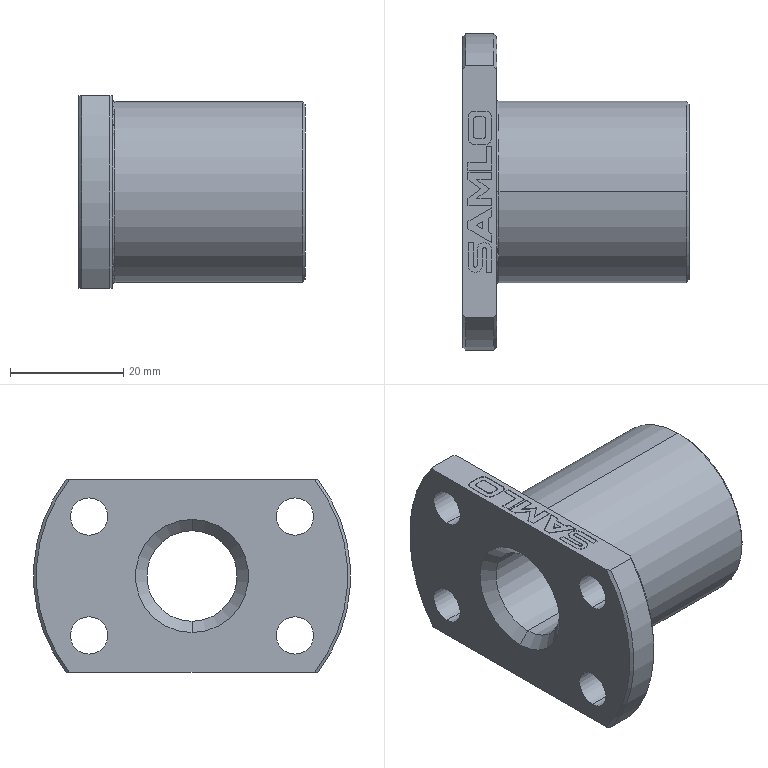Part | SolidWorks | features BaseBody 1 | 1 solid | 95 faces | box 40 x 56 x 34 mm | volume 28906 mm3 | plane 57 | cylinder 26 | cone 10 | torus 2 | commonest cylinder face diameters 6.6 x8 0.965 x4 2.045 x4 0.692 x2 2.535 x2 16 x2